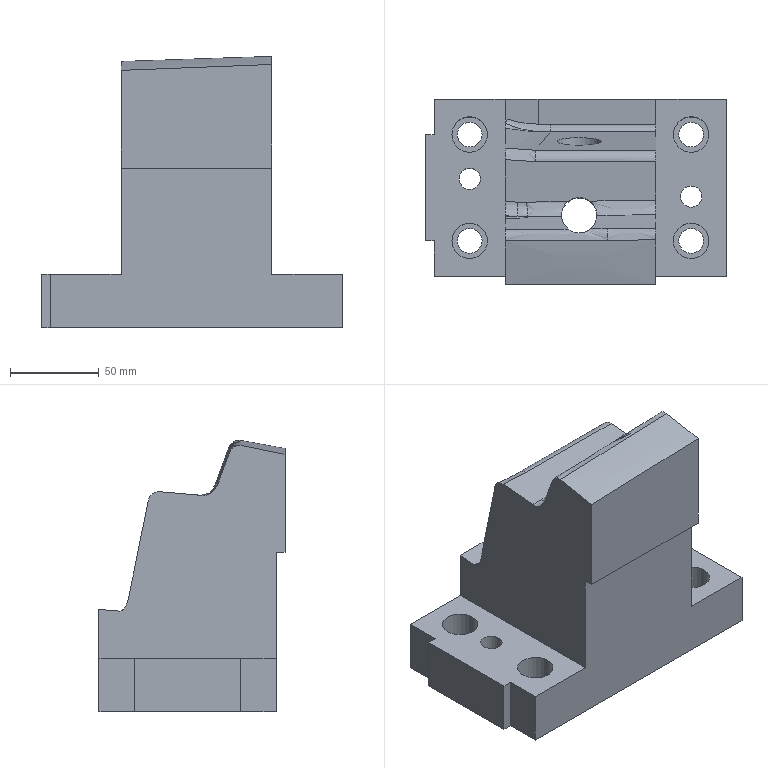Part | NX | features solid 2 | 1 solid | 56 faces | box 170 x 105 x 153.114 mm | volume 1167272 mm3 | spline 22 | plane 20 | cylinder 14 | commonest cylinder face diameters 20 x5 14 x4 12 x2 4 x1 18.6 x1 25 x1